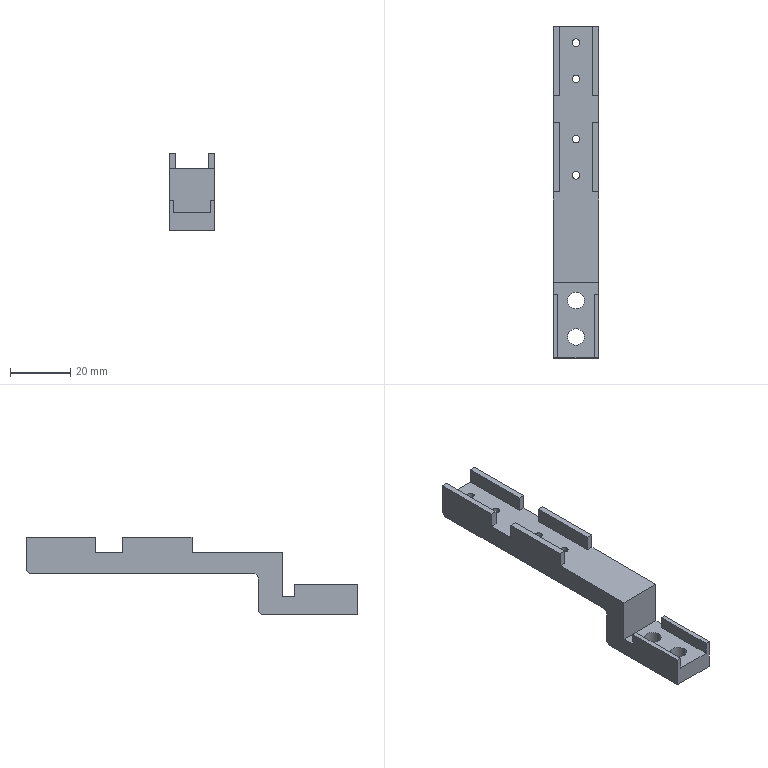Part | STEP file | 2040 Cylinder material clamp B | 1 solid | 45 faces | box 15 x 110 x 25.8 mm | volume 13578 mm3 | plane 32 | cylinder 13 | commonest cylinder face diameters 2.5 x8 5.5 x4 4 x1